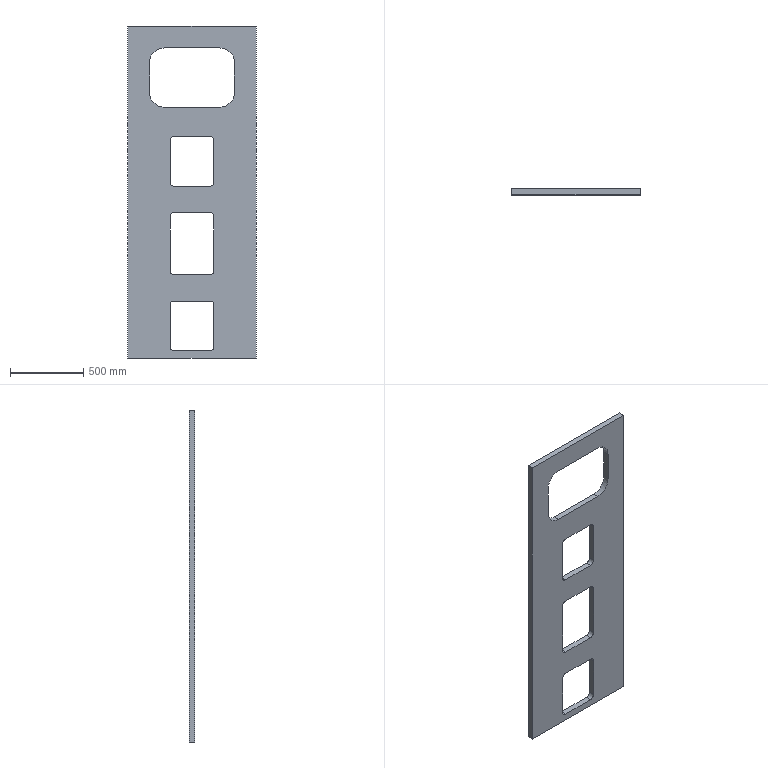Part | SolidWorks | features Cut 4, Fillet 2, Extrusion 1 | 1 solid | 38 faces | box 880 x 40 x 2266 mm | volume 57536483 mm3 | plane 22 | cylinder 16 | commonest cylinder face diameters 60 x12 200 x4
STEP:
#1=CARTESIAN_POINT('',(440.,0.,1133.));
#2=VERTEX_POINT('',#1);
#3=CARTESIAN_POINT('',(440.,0.,-1133.));
#4=VERTEX_POINT('',#3);
#5=CARTESIAN_POINT('',(440.,0.,1133.));
#6=DIRECTION('',(0.,0.,-1.));
#7=VECTOR('',#6,1000.);
#8=LINE('',#5,#7);
#9=EDGE_CURVE('',#2,#4,#8,.T.);
#10=ORIENTED_EDGE('',*,*,#9,.T.);
#11=CARTESIAN_POINT('',(440.,40.,-1133.));
#12=VERTEX_POINT('',#11);
#13=CARTESIAN_POINT('',(440.,40.,-1133.));
#14=DIRECTION('',(0.,-1.,0.));
#15=VECTOR('',#14,1000.);
#16=LINE('',#13,#15);
#17=EDGE_CURVE('',#12,#4,#16,.T.);
#18=ORIENTED_EDGE('',*,*,#17,.F.);
#19=CARTESIAN_POINT('',(440.,40.,1133.));
#20=VERTEX_POINT('',#19);
#21=CARTESIAN_POINT('',(440.,40.,1133.));
#22=DIRECTION('',(0.,0.,-1.));
#23=VECTOR('',#22,1000.);
#24=LINE('',#21,#23);
#25=EDGE_CURVE('',#20,#12,#24,.T.);
#26=ORIENTED_EDGE('',*,*,#25,.F.);
#27=CARTESIAN_POINT('',(440.,40.,1133.));
#28=DIRECTION('',(0.,-1.,0.));
#29=VECTOR('',#28,1000.);
#30=LINE('',#27,#29);
#31=EDGE_CURVE('',#20,#2,#30,.T.);
#32=ORIENTED_EDGE('',*,*,#31,.T.);
#33=EDGE_LOOP('',(#10,#18,#26,#32));
#34=FACE_OUTER_BOUND('',#33,.T.);
#35=CARTESIAN_POINT('',(440.,40.,1133.));
#36=DIRECTION('',(-1.,0.,0.));
#37=DIRECTION('',(0.,0.,1.));
#38=AXIS2_PLACEMENT_3D('',#35,#36,#37);
#39=PLANE('',#38);
#40=ADVANCED_FACE('',(#34),#39,.F.);
#41=CARTESIAN_POINT('',(-440.,0.,-1133.));
#42=VERTEX_POINT('',#41);
#43=CARTESIAN_POINT('',(-440.,0.,-1133.));
#44=DIRECTION('',(-1.,0.,0.));
#45=VECTOR('',#44,1000.);
#46=LINE('',#43,#45);
#47=EDGE_CURVE('',#4,#42,#46,.T.);
#48=ORIENTED_EDGE('',*,*,#47,.T.);
#49=CARTESIAN_POINT('',(-440.,40.,-1133.));
#50=VERTEX_POINT('',#49);
#51=CARTESIAN_POINT('',(-440.,40.,-1133.));
#52=DIRECTION('',(0.,-1.,0.));
#53=VECTOR('',#52,1000.);
#54=LINE('',#51,#53);
#55=EDGE_CURVE('',#50,#42,#54,.T.);
#56=ORIENTED_EDGE('',*,*,#55,.F.);
#57=CARTESIAN_POINT('',(-440.,40.,-1133.));
#58=DIRECTION('',(-1.,0.,0.));
#59=VECTOR('',#58,1000.);
#60=LINE('',#57,#59);
#61=EDGE_CURVE('',#12,#50,#60,.T.);
#62=ORIENTED_EDGE('',*,*,#61,.F.);
#63=ORIENTED_EDGE('',*,*,#17,.T.);
#64=EDGE_LOOP('',(#48,#56,#62,#63));
#65=FACE_OUTER_BOUND('',#64,.T.);
#66=CARTESIAN_POINT('',(-440.,40.,-1133.));
#67=DIRECTION('',(0.,0.,1.));
#68=DIRECTION('',(1.,0.,0.));
#69=AXIS2_PLACEMENT_3D('',#66,#67,#68);
#70=PLANE('',#69);
#71=ADVANCED_FACE('',(#65),#70,.F.);
#72=CARTESIAN_POINT('',(-440.,0.,1133.));
#73=VERTEX_POINT('',#72);
#74=CARTESIAN_POINT('',(-440.,0.,1133.));
#75=DIRECTION('',(0.,0.,1.));
#76=VECTOR('',#75,1000.);
#77=LINE('',#74,#76);
#78=EDGE_CURVE('',#42,#73,#77,.T.);
#79=ORIENTED_EDGE('',*,*,#78,.T.);
#80=CARTESIAN_POINT('',(-440.,40.,1133.));
#81=VERTEX_POINT('',#80);
#82=CARTESIAN_POINT('',(-440.,40.,1133.));
#83=DIRECTION('',(0.,-1.,0.));
#84=VECTOR('',#83,1000.);
#85=LINE('',#82,#84);
#86=EDGE_CURVE('',#81,#73,#85,.T.);
#87=ORIENTED_EDGE('',*,*,#86,.F.);
#88=CARTESIAN_POINT('',(-440.,40.,1133.));
#89=DIRECTION('',(0.,0.,1.));
#90=VECTOR('',#89,1000.);
#91=LINE('',#88,#90);
#92=EDGE_CURVE('',#50,#81,#91,.T.);
#93=ORIENTED_EDGE('',*,*,#92,.F.);
#94=ORIENTED_EDGE('',*,*,#55,.T.);
#95=EDGE_LOOP('',(#79,#87,#93,#94));
#96=FACE_OUTER_BOUND('',#95,.T.);
#97=CARTESIAN_POINT('',(-440.,40.,1133.));
#98=DIRECTION('',(1.,0.,0.));
#99=DIRECTION('',(0.,0.,-1.));
#100=AXIS2_PLACEMENT_3D('',#97,#98,#99);
#101=PLANE('',#100);
#102=ADVANCED_FACE('',(#96),#101,.F.);
#103=CARTESIAN_POINT('',(-440.,0.,1133.));
#104=DIRECTION('',(1.,0.,0.));
#105=VECTOR('',#104,1000.);
#106=LINE('',#103,#105);
#107=EDGE_CURVE('',#73,#2,#106,.T.);
#108=ORIENTED_EDGE('',*,*,#107,.T.);
#109=ORIENTED_EDGE('',*,*,#31,.F.);
#110=CARTESIAN_POINT('',(-440.,40.,1133.));
#111=DIRECTION('',(1.,0.,0.));
#112=VECTOR('',#111,1000.);
#113=LINE('',#110,#112);
#114=EDGE_CURVE('',#81,#20,#113,.T.);
#115=ORIENTED_EDGE('',*,*,#114,.F.);
#116=ORIENTED_EDGE('',*,*,#86,.T.);
#117=EDGE_LOOP('',(#108,#109,#115,#116));
#118=FACE_OUTER_BOUND('',#117,.T.);
#119=CARTESIAN_POINT('',(-440.,40.,1133.));
#120=DIRECTION('',(0.,0.,-1.));
#121=DIRECTION('',(-1.,0.,0.));
#122=AXIS2_PLACEMENT_3D('',#119,#120,#121);
#123=PLANE('',#122);
#124=ADVANCED_FACE('',(#118),#123,.F.);
#125=CARTESIAN_POINT('',(290.,40.,678.985));
#126=VERTEX_POINT('',#125);
#127=CARTESIAN_POINT('',(290.,40.,883.));
#128=VERTEX_POINT('',#127);
#129=CARTESIAN_POINT('',(290.,40.,983.));
#130=DIRECTION('',(0.,0.,1.));
#131=VECTOR('',#130,1000.);
#132=LINE('',#129,#131);
#133=EDGE_CURVE('',#126,#128,#132,.T.);
#134=ORIENTED_EDGE('',*,*,#133,.T.);
#135=CARTESIAN_POINT('',(190.,40.,983.));
#136=VERTEX_POINT('',#135);
#137=CARTESIAN_POINT('',(190.,40.,883.));
#138=DIRECTION('',(0.,-1.,0.));
#139=DIRECTION('',(0.,0.,-1.));
#140=AXIS2_PLACEMENT_3D('',#137,#138,#139);
#141=CIRCLE('',#140,100.);
#142=EDGE_CURVE('',#128,#136,#141,.T.);
#143=ORIENTED_EDGE('',*,*,#142,.T.);
#144=CARTESIAN_POINT('',(-190.,40.,983.));
#145=VERTEX_POINT('',#144);
#146=CARTESIAN_POINT('',(-290.,40.,983.));
#147=DIRECTION('',(-1.,0.,0.));
#148=VECTOR('',#147,1000.);
#149=LINE('',#146,#148);
#150=EDGE_CURVE('',#136,#145,#149,.T.);
#151=ORIENTED_EDGE('',*,*,#150,.T.);
#152=CARTESIAN_POINT('',(-290.,40.,883.));
#153=VERTEX_POINT('',#152);
#154=CARTESIAN_POINT('',(-190.,40.,883.));
#155=DIRECTION('',(0.,-1.,0.));
#156=DIRECTION('',(0.,0.,-1.));
#157=AXIS2_PLACEMENT_3D('',#154,#155,#156);
#158=CIRCLE('',#157,100.);
#159=EDGE_CURVE('',#145,#153,#158,.T.);
#160=ORIENTED_EDGE('',*,*,#159,.T.);
#161=CARTESIAN_POINT('',(-290.,40.,678.985));
#162=VERTEX_POINT('',#161);
#163=CARTESIAN_POINT('',(-290.,40.,983.));
#164=DIRECTION('',(0.,0.,-1.));
#165=VECTOR('',#164,1000.);
#166=LINE('',#163,#165);
#167=EDGE_CURVE('',#153,#162,#166,.T.);
#168=ORIENTED_EDGE('',*,*,#167,.T.);
#169=CARTESIAN_POINT('',(-190.,40.,578.985));
#170=VERTEX_POINT('',#169);
#171=CARTESIAN_POINT('',(-190.,40.,678.985));
#172=DIRECTION('',(0.,-1.,0.));
#173=DIRECTION('',(0.,0.,-1.));
#174=AXIS2_PLACEMENT_3D('',#171,#172,#173);
#175=CIRCLE('',#174,100.);
#176=EDGE_CURVE('',#162,#170,#175,.T.);
#177=ORIENTED_EDGE('',*,*,#176,.T.);
#178=CARTESIAN_POINT('',(190.,40.,578.985));
#179=VERTEX_POINT('',#178);
#180=CARTESIAN_POINT('',(-290.,40.,578.985));
#181=DIRECTION('',(1.,0.,0.));
#182=VECTOR('',#181,1000.);
#183=LINE('',#180,#182);
#184=EDGE_CURVE('',#170,#179,#183,.T.);
#185=ORIENTED_EDGE('',*,*,#184,.T.);
#186=CARTESIAN_POINT('',(190.,40.,678.985));
#187=DIRECTION('',(0.,-1.,0.));
#188=DIRECTION('',(0.,0.,-1.));
#189=AXIS2_PLACEMENT_3D('',#186,#187,#188);
#190=CIRCLE('',#189,100.);
#191=EDGE_CURVE('',#179,#126,#190,.T.);
#192=ORIENTED_EDGE('',*,*,#191,.T.);
#193=EDGE_LOOP('',(#134,#143,#151,#160,#168,#177,#185,#192));
#194=FACE_BOUND('',#193,.T.);
#195=CARTESIAN_POINT('',(150.,40.,-1054.485));
#196=VERTEX_POINT('',#195);
#197=CARTESIAN_POINT('',(150.,40.,-774.015));
#198=VERTEX_POINT('',#197);
#199=CARTESIAN_POINT('',(150.,40.,-744.015));
#200=DIRECTION('',(0.,0.,1.));
#201=VECTOR('',#200,1000.);
#202=LINE('',#199,#201);
#203=EDGE_CURVE('',#196,#198,#202,.T.);
#204=ORIENTED_EDGE('',*,*,#203,.T.);
#205=CARTESIAN_POINT('',(120.,40.,-744.015));
#206=VERTEX_POINT('',#205);
#207=CARTESIAN_POINT('',(120.,40.,-774.015));
#208=DIRECTION('',(0.,-1.,0.));
#209=DIRECTION('',(0.,0.,-1.));
#210=AXIS2_PLACEMENT_3D('',#207,#208,#209);
#211=CIRCLE('',#210,30.);
#212=EDGE_CURVE('',#198,#206,#211,.T.);
#213=ORIENTED_EDGE('',*,*,#212,.T.);
#214=CARTESIAN_POINT('',(-120.,40.,-744.015));
#215=VERTEX_POINT('',#214);
#216=CARTESIAN_POINT('',(-150.,40.,-744.015));
#217=DIRECTION('',(-1.,0.,0.));
#218=VECTOR('',#217,1000.);
#219=LINE('',#216,#218);
#220=EDGE_CURVE('',#206,#215,#219,.T.);
#221=ORIENTED_EDGE('',*,*,#220,.T.);
#222=CARTESIAN_POINT('',(-150.,40.,-774.015));
#223=VERTEX_POINT('',#222);
#224=CARTESIAN_POINT('',(-120.,40.,-774.015));
#225=DIRECTION('',(0.,-1.,0.));
#226=DIRECTION('',(0.,0.,-1.));
#227=AXIS2_PLACEMENT_3D('',#224,#225,#226);
#228=CIRCLE('',#227,30.);
#229=EDGE_CURVE('',#215,#223,#228,.T.);
#230=ORIENTED_EDGE('',*,*,#229,.T.);
#231=CARTESIAN_POINT('',(-150.,40.,-1054.485));
#232=VERTEX_POINT('',#231);
#233=CARTESIAN_POINT('',(-150.,40.,-744.015));
#234=DIRECTION('',(0.,0.,-1.));
#235=VECTOR('',#234,1000.);
#236=LINE('',#233,#235);
#237=EDGE_CURVE('',#223,#232,#236,.T.);
#238=ORIENTED_EDGE('',*,*,#237,.T.);
#239=CARTESIAN_POINT('',(-120.,40.,-1084.485));
#240=VERTEX_POINT('',#239);
#241=CARTESIAN_POINT('',(-120.,40.,-1054.485));
#242=DIRECTION('',(0.,-1.,0.));
#243=DIRECTION('',(0.,0.,-1.));
#244=AXIS2_PLACEMENT_3D('',#241,#242,#243);
#245=CIRCLE('',#244,30.);
#246=EDGE_CURVE('',#232,#240,#245,.T.);
#247=ORIENTED_EDGE('',*,*,#246,.T.);
#248=CARTESIAN_POINT('',(120.,40.,-1084.485));
#249=VERTEX_POINT('',#248);
#250=CARTESIAN_POINT('',(-150.,40.,-1084.485));
#251=DIRECTION('',(1.,0.,0.));
#252=VECTOR('',#251,1000.);
#253=LINE('',#250,#252);
#254=EDGE_CURVE('',#240,#249,#253,.T.);
#255=ORIENTED_EDGE('',*,*,#254,.T.);
#256=CARTESIAN_POINT('',(120.,40.,-1054.485));
#257=DIRECTION('',(0.,-1.,0.));
#258=DIRECTION('',(0.,0.,-1.));
#259=AXIS2_PLACEMENT_3D('',#256,#257,#258);
#260=CIRCLE('',#259,30.);
#261=EDGE_CURVE('',#249,#196,#260,.T.);
#262=ORIENTED_EDGE('',*,*,#261,.T.);
#263=EDGE_LOOP('',(#204,#213,#221,#230,#238,#247,#255,#262));
#264=FACE_BOUND('',#263,.T.);
#265=CARTESIAN_POINT('',(150.,40.,-536.015));
#266=VERTEX_POINT('',#265);
#267=CARTESIAN_POINT('',(150.,40.,-169.485));
#268=VERTEX_POINT('',#267);
#269=CARTESIAN_POINT('',(150.,40.,-566.015));
#270=DIRECTION('',(0.,0.,1.));
#271=VECTOR('',#270,1000.);
#272=LINE('',#269,#271);
#273=EDGE_CURVE('',#266,#268,#272,.T.);
#274=ORIENTED_EDGE('',*,*,#273,.T.);
#275=CARTESIAN_POINT('',(120.,40.,-139.485));
#276=VERTEX_POINT('',#275);
#277=CARTESIAN_POINT('',(120.,40.,-169.485));
#278=DIRECTION('',(0.,-1.,0.));
#279=DIRECTION('',(0.,0.,-1.));
#280=AXIS2_PLACEMENT_3D('',#277,#278,#279);
#281=CIRCLE('',#280,30.);
#282=EDGE_CURVE('',#268,#276,#281,.T.);
#283=ORIENTED_EDGE('',*,*,#282,.T.);
#284=CARTESIAN_POINT('',(-120.,40.,-139.485));
#285=VERTEX_POINT('',#284);
#286=CARTESIAN_POINT('',(-150.,40.,-139.485));
#287=DIRECTION('',(-1.,0.,0.));
#288=VECTOR('',#287,1000.);
#289=LINE('',#286,#288);
#290=EDGE_CURVE('',#276,#285,#289,.T.);
#291=ORIENTED_EDGE('',*,*,#290,.T.);
#292=CARTESIAN_POINT('',(-150.,40.,-169.485));
#293=VERTEX_POINT('',#292);
#294=CARTESIAN_POINT('',(-120.,40.,-169.485));
#295=DIRECTION('',(0.,-1.,0.));
#296=DIRECTION('',(0.,0.,-1.));
#297=AXIS2_PLACEMENT_3D('',#294,#295,#296);
#298=CIRCLE('',#297,30.);
#299=EDGE_CURVE('',#285,#293,#298,.T.);
#300=ORIENTED_EDGE('',*,*,#299,.T.);
#301=CARTESIAN_POINT('',(-150.,40.,-536.015));
#302=VERTEX_POINT('',#301);
#303=CARTESIAN_POINT('',(-150.,40.,-566.015));
#304=DIRECTION('',(0.,0.,-1.));
#305=VECTOR('',#304,1000.);
#306=LINE('',#303,#305);
#307=EDGE_CURVE('',#293,#302,#306,.T.);
#308=ORIENTED_EDGE('',*,*,#307,.T.);
#309=CARTESIAN_POINT('',(-120.,40.,-566.015));
#310=VERTEX_POINT('',#309);
#311=CARTESIAN_POINT('',(-120.,40.,-536.015));
#312=DIRECTION('',(0.,-1.,0.));
#313=DIRECTION('',(0.,0.,-1.));
#314=AXIS2_PLACEMENT_3D('',#311,#312,#313);
#315=CIRCLE('',#314,30.);
#316=EDGE_CURVE('',#302,#310,#315,.T.);
#317=ORIENTED_EDGE('',*,*,#316,.T.);
#318=CARTESIAN_POINT('',(120.,40.,-566.015));
#319=VERTEX_POINT('',#318);
#320=CARTESIAN_POINT('',(-150.,40.,-566.015));
#321=DIRECTION('',(1.,0.,0.));
#322=VECTOR('',#321,1000.);
#323=LINE('',#320,#322);
#324=EDGE_CURVE('',#310,#319,#323,.T.);
#325=ORIENTED_EDGE('',*,*,#324,.T.);
#326=CARTESIAN_POINT('',(120.,40.,-536.015));
#327=DIRECTION('',(0.,-1.,0.));
#328=DIRECTION('',(0.,0.,-1.));
#329=AXIS2_PLACEMENT_3D('',#326,#327,#328);
#330=CIRCLE('',#329,30.);
#331=EDGE_CURVE('',#319,#266,#330,.T.);
#332=ORIENTED_EDGE('',*,*,#331,.T.);
#333=EDGE_LOOP('',(#274,#283,#291,#300,#308,#317,#325,#332));
#334=FACE_BOUND('',#333,.T.);
#335=CARTESIAN_POINT('',(150.,40.,68.515));
#336=VERTEX_POINT('',#335);
#337=CARTESIAN_POINT('',(150.,40.,348.985));
#338=VERTEX_POINT('',#337);
#339=CARTESIAN_POINT('',(150.,40.,378.985));
#340=DIRECTION('',(0.,0.,1.));
#341=VECTOR('',#340,1000.);
#342=LINE('',#339,#341);
#343=EDGE_CURVE('',#336,#338,#342,.T.);
#344=ORIENTED_EDGE('',*,*,#343,.T.);
#345=CARTESIAN_POINT('',(120.,40.,378.985));
#346=VERTEX_POINT('',#345);
#347=CARTESIAN_POINT('',(120.,40.,348.985));
#348=DIRECTION('',(0.,-1.,0.));
#349=DIRECTION('',(0.,0.,-1.));
#350=AXIS2_PLACEMENT_3D('',#347,#348,#349);
#351=CIRCLE('',#350,30.);
#352=EDGE_CURVE('',#338,#346,#351,.T.);
#353=ORIENTED_EDGE('',*,*,#352,.T.);
#354=CARTESIAN_POINT('',(-120.,40.,378.985));
#355=VERTEX_POINT('',#354);
#356=CARTESIAN_POINT('',(-150.,40.,378.985));
#357=DIRECTION('',(-1.,0.,0.));
#358=VECTOR('',#357,1000.);
#359=LINE('',#356,#358);
#360=EDGE_CURVE('',#346,#355,#359,.T.);
#361=ORIENTED_EDGE('',*,*,#360,.T.);
#362=CARTESIAN_POINT('',(-150.,40.,348.985));
#363=VERTEX_POINT('',#362);
#364=CARTESIAN_POINT('',(-120.,40.,348.985));
#365=DIRECTION('',(0.,-1.,0.));
#366=DIRECTION('',(0.,0.,-1.));
#367=AXIS2_PLACEMENT_3D('',#364,#365,#366);
#368=CIRCLE('',#367,30.);
#369=EDGE_CURVE('',#355,#363,#368,.T.);
#370=ORIENTED_EDGE('',*,*,#369,.T.);
#371=CARTESIAN_POINT('',(-150.,40.,68.515));
#372=VERTEX_POINT('',#371);
#373=CARTESIAN_POINT('',(-150.,40.,378.985));
#374=DIRECTION('',(0.,0.,-1.));
#375=VECTOR('',#374,1000.);
#376=LINE('',#373,#375);
#377=EDGE_CURVE('',#363,#372,#376,.T.);
#378=ORIENTED_EDGE('',*,*,#377,.T.);
#379=CARTESIAN_POINT('',(-120.,40.,38.515));
#380=VERTEX_POINT('',#379);
#381=CARTESIAN_POINT('',(-120.,40.,68.515));
#382=DIRECTION('',(0.,-1.,0.));
#383=DIRECTION('',(0.,0.,-1.));
#384=AXIS2_PLACEMENT_3D('',#381,#382,#383);
#385=CIRCLE('',#384,30.);
#386=EDGE_CURVE('',#372,#380,#385,.T.);
#387=ORIENTED_EDGE('',*,*,#386,.T.);
#388=CARTESIAN_POINT('',(120.,40.,38.515));
#389=VERTEX_POINT('',#388);
#390=CARTESIAN_POINT('',(-150.,40.,38.515));
#391=DIRECTION('',(1.,0.,0.));
#392=VECTOR('',#391,1000.);
#393=LINE('',#390,#392);
#394=EDGE_CURVE('',#380,#389,#393,.T.);
#395=ORIENTED_EDGE('',*,*,#394,.T.);
#396=CARTESIAN_POINT('',(120.,40.,68.515));
#397=DIRECTION('',(0.,-1.,0.));
#398=DIRECTION('',(0.,0.,-1.));
#399=AXIS2_PLACEMENT_3D('',#396,#397,#398);
#400=CIRCLE('',#399,30.);
#401=EDGE_CURVE('',#389,#336,#400,.T.);
#402=ORIENTED_EDGE('',*,*,#401,.T.);
#403=EDGE_LOOP('',(#344,#353,#361,#370,#378,#387,#395,#402));
#404=FACE_BOUND('',#403,.T.);
#405=ORIENTED_EDGE('',*,*,#25,.T.);
#406=ORIENTED_EDGE('',*,*,#61,.T.);
#407=ORIENTED_EDGE('',*,*,#92,.T.);
#408=ORIENTED_EDGE('',*,*,#114,.T.);
#409=EDGE_LOOP('',(#405,#406,#407,#408));
#410=FACE_OUTER_BOUND('',#409,.T.);
#411=CARTESIAN_POINT('',(0.,40.,0.));
#412=DIRECTION('',(0.,-1.,0.));
#413=DIRECTION('',(0.,0.,-1.));
#414=AXIS2_PLACEMENT_3D('',#411,#412,#413);
#415=PLANE('',#414);
#416=ADVANCED_FACE('',(#194,#264,#334,#404,#410),#415,.F.);
#417=CARTESIAN_POINT('',(-290.,0.,883.));
#418=VERTEX_POINT('',#417);
#419=CARTESIAN_POINT('',(-290.,0.,678.985));
#420=VERTEX_POINT('',#419);
#421=CARTESIAN_POINT('',(-290.,0.,983.));
#422=DIRECTION('',(0.,0.,-1.));
#423=VECTOR('',#422,1000.);
#424=LINE('',#421,#423);
#425=EDGE_CURVE('',#418,#420,#424,.T.);
#426=ORIENTED_EDGE('',*,*,#425,.F.);
#427=CARTESIAN_POINT('',(-190.,0.,983.));
#428=VERTEX_POINT('',#427);
#429=CARTESIAN_POINT('',(-190.,0.,883.));
#430=DIRECTION('',(0.,1.,0.));
#431=DIRECTION('',(0.,0.,-1.));
#432=AXIS2_PLACEMENT_3D('',#429,#430,#431);
#433=CIRCLE('',#432,100.);
#434=EDGE_CURVE('',#418,#428,#433,.T.);
#435=ORIENTED_EDGE('',*,*,#434,.T.);
#436=CARTESIAN_POINT('',(190.,0.,983.));
#437=VERTEX_POINT('',#436);
#438=CARTESIAN_POINT('',(-290.,0.,983.));
#439=DIRECTION('',(-1.,0.,0.));
#440=VECTOR('',#439,1000.);
#441=LINE('',#438,#440);
#442=EDGE_CURVE('',#437,#428,#441,.T.);
#443=ORIENTED_EDGE('',*,*,#442,.F.);
#444=CARTESIAN_POINT('',(290.,0.,883.));
#445=VERTEX_POINT('',#444);
#446=CARTESIAN_POINT('',(190.,0.,883.));
#447=DIRECTION('',(0.,1.,0.));
#448=DIRECTION('',(0.,0.,-1.));
#449=AXIS2_PLACEMENT_3D('',#446,#447,#448);
#450=CIRCLE('',#449,100.);
#451=EDGE_CURVE('',#437,#445,#450,.T.);
#452=ORIENTED_EDGE('',*,*,#451,.T.);
#453=CARTESIAN_POINT('',(290.,0.,678.985));
#454=VERTEX_POINT('',#453);
#455=CARTESIAN_POINT('',(290.,0.,983.));
#456=DIRECTION('',(0.,0.,1.));
#457=VECTOR('',#456,1000.);
#458=LINE('',#455,#457);
#459=EDGE_CURVE('',#454,#445,#458,.T.);
#460=ORIENTED_EDGE('',*,*,#459,.F.);
#461=CARTESIAN_POINT('',(190.,0.,578.985));
#462=VERTEX_POINT('',#461);
#463=CARTESIAN_POINT('',(190.,0.,678.985));
#464=DIRECTION('',(0.,1.,0.));
#465=DIRECTION('',(0.,0.,-1.));
#466=AXIS2_PLACEMENT_3D('',#463,#464,#465);
#467=CIRCLE('',#466,100.);
#468=EDGE_CURVE('',#454,#462,#467,.T.);
#469=ORIENTED_EDGE('',*,*,#468,.T.);
#470=CARTESIAN_POINT('',(-190.,0.,578.985));
#471=VERTEX_POINT('',#470);
#472=CARTESIAN_POINT('',(-290.,0.,578.985));
#473=DIRECTION('',(1.,0.,0.));
#474=VECTOR('',#473,1000.);
#475=LINE('',#472,#474);
#476=EDGE_CURVE('',#471,#462,#475,.T.);
#477=ORIENTED_EDGE('',*,*,#476,.F.);
#478=CARTESIAN_POINT('',(-190.,0.,678.985));
#479=DIRECTION('',(0.,1.,0.));
#480=DIRECTION('',(0.,0.,-1.));
#481=AXIS2_PLACEMENT_3D('',#478,#479,#480);
#482=CIRCLE('',#481,100.);
#483=EDGE_CURVE('',#471,#420,#482,.T.);
#484=ORIENTED_EDGE('',*,*,#483,.T.);
#485=EDGE_LOOP('',(#426,#435,#443,#452,#460,#469,#477,#484));
#486=FACE_BOUND('',#485,.T.);
#487=CARTESIAN_POINT('',(-150.,0.,-774.015));
#488=VERTEX_POINT('',#487);
#489=CARTESIAN_POINT('',(-150.,0.,-1054.485));
#490=VERTEX_POINT('',#489);
#491=CARTESIAN_POINT('',(-150.,0.,-744.015));
#492=DIRECTION('',(0.,0.,-1.));
#493=VECTOR('',#492,1000.);
#494=LINE('',#491,#493);
#495=EDGE_CURVE('',#488,#490,#494,.T.);
#496=ORIENTED_EDGE('',*,*,#495,.F.);
#497=CARTESIAN_POINT('',(-120.,0.,-744.015));
#498=VERTEX_POINT('',#497);
#499=CARTESIAN_POINT('',(-120.,0.,-774.015));
#500=DIRECTION('',(0.,1.,0.));
#501=DIRECTION('',(0.,0.,-1.));
#502=AXIS2_PLACEMENT_3D('',#499,#500,#501);
#503=CIRCLE('',#502,30.);
#504=EDGE_CURVE('',#488,#498,#503,.T.);
#505=ORIENTED_EDGE('',*,*,#504,.T.);
#506=CARTESIAN_POINT('',(120.,0.,-744.015));
#507=VERTEX_POINT('',#506);
#508=CARTESIAN_POINT('',(-150.,0.,-744.015));
#509=DIRECTION('',(-1.,0.,0.));
#510=VECTOR('',#509,1000.);
#511=LINE('',#508,#510);
#512=EDGE_CURVE('',#507,#498,#511,.T.);
#513=ORIENTED_EDGE('',*,*,#512,.F.);
#514=CARTESIAN_POINT('',(150.,0.,-774.015));
#515=VERTEX_POINT('',#514);
#516=CARTESIAN_POINT('',(120.,0.,-774.015));
#517=DIRECTION('',(0.,1.,0.));
#518=DIRECTION('',(0.,0.,-1.));
#519=AXIS2_PLACEMENT_3D('',#516,#517,#518);
#520=CIRCLE('',#519,30.);
#521=EDGE_CURVE('',#507,#515,#520,.T.);
#522=ORIENTED_EDGE('',*,*,#521,.T.);
#523=CARTESIAN_POINT('',(150.,0.,-1054.485));
#524=VERTEX_POINT('',#523);
#525=CARTESIAN_POINT('',(150.,0.,-744.015));
#526=DIRECTION('',(0.,0.,1.));
#527=VECTOR('',#526,1000.);
#528=LINE('',#525,#527);
#529=EDGE_CURVE('',#524,#515,#528,.T.);
#530=ORIENTED_EDGE('',*,*,#529,.F.);
#531=CARTESIAN_POINT('',(120.,0.,-1084.485));
#532=VERTEX_POINT('',#531);
#533=CARTESIAN_POINT('',(120.,0.,-1054.485));
#534=DIRECTION('',(0.,1.,0.));
#535=DIRECTION('',(0.,0.,-1.));
#536=AXIS2_PLACEMENT_3D('',#533,#534,#535);
#537=CIRCLE('',#536,30.);
#538=EDGE_CURVE('',#524,#532,#537,.T.);
#539=ORIENTED_EDGE('',*,*,#538,.T.);
#540=CARTESIAN_POINT('',(-120.,0.,-1084.485));
#541=VERTEX_POINT('',#540);
#542=CARTESIAN_POINT('',(-150.,0.,-1084.485));
#543=DIRECTION('',(1.,0.,0.));
#544=VECTOR('',#543,1000.);
#545=LINE('',#542,#544);
#546=EDGE_CURVE('',#541,#532,#545,.T.);
#547=ORIENTED_EDGE('',*,*,#546,.F.);
#548=CARTESIAN_POINT('',(-120.,0.,-1054.485));
#549=DIRECTION('',(0.,1.,0.));
#550=DIRECTION('',(0.,0.,-1.));
#551=AXIS2_PLACEMENT_3D('',#548,#549,#550);
#552=CIRCLE('',#551,30.);
#553=EDGE_CURVE('',#541,#490,#552,.T.);
#554=ORIENTED_EDGE('',*,*,#553,.T.);
#555=EDGE_LOOP('',(#496,#505,#513,#522,#530,#539,#547,#554));
#556=FACE_BOUND('',#555,.T.);
#557=CARTESIAN_POINT('',(-150.,0.,-169.485));
#558=VERTEX_POINT('',#557);
#559=CARTESIAN_POINT('',(-150.,0.,-536.015));
#560=VERTEX_POINT('',#559);
#561=CARTESIAN_POINT('',(-150.,0.,-566.015));
#562=DIRECTION('',(0.,0.,-1.));
#563=VECTOR('',#562,1000.);
#564=LINE('',#561,#563);
#565=EDGE_CURVE('',#558,#560,#564,.T.);
#566=ORIENTED_EDGE('',*,*,#565,.F.);
#567=CARTESIAN_POINT('',(-120.,0.,-139.485));
#568=VERTEX_POINT('',#567);
#569=CARTESIAN_POINT('',(-120.,0.,-169.485));
#570=DIRECTION('',(0.,1.,0.));
#571=DIRECTION('',(0.,0.,-1.));
#572=AXIS2_PLACEMENT_3D('',#569,#570,#571);
#573=CIRCLE('',#572,30.);
#574=EDGE_CURVE('',#558,#568,#573,.T.);
#575=ORIENTED_EDGE('',*,*,#574,.T.);
#576=CARTESIAN_POINT('',(120.,0.,-139.485));
#577=VERTEX_POINT('',#576);
#578=CARTESIAN_POINT('',(-150.,0.,-139.485));
#579=DIRECTION('',(-1.,0.,0.));
#580=VECTOR('',#579,1000.);
#581=LINE('',#578,#580);
#582=EDGE_CURVE('',#577,#568,#581,.T.);
#583=ORIENTED_EDGE('',*,*,#582,.F.);
#584=CARTESIAN_POINT('',(150.,0.,-169.485));
#585=VERTEX_POINT('',#584);
#586=CARTESIAN_POINT('',(120.,0.,-169.485));
#587=DIRECTION('',(0.,1.,0.));
#588=DIRECTION('',(0.,0.,-1.));
#589=AXIS2_PLACEMENT_3D('',#586,#587,#588);
#590=CIRCLE('',#589,30.);
#591=EDGE_CURVE('',#577,#585,#590,.T.);
#592=ORIENTED_EDGE('',*,*,#591,.T.);
#593=CARTESIAN_POINT('',(150.,0.,-536.015));
#594=VERTEX_POINT('',#593);
#595=CARTESIAN_POINT('',(150.,0.,-566.015));
#596=DIRECTION('',(0.,0.,1.));
#597=VECTOR('',#596,1000.);
#598=LINE('',#595,#597);
#599=EDGE_CURVE('',#594,#585,#598,.T.);
#600=ORIENTED_EDGE('',*,*,#599,.F.);
#601=CARTESIAN_POINT('',(120.,0.,-566.015));
#602=VERTEX_POINT('',#601);
#603=CARTESIAN_POINT('',(120.,0.,-536.015));
#604=DIRECTION('',(0.,1.,0.));
#605=DIRECTION('',(0.,0.,-1.));
#606=AXIS2_PLACEMENT_3D('',#603,#604,#605);
#607=CIRCLE('',#606,30.);
#608=EDGE_CURVE('',#594,#602,#607,.T.);
#609=ORIENTED_EDGE('',*,*,#608,.T.);
#610=CARTESIAN_POINT('',(-120.,0.,-566.015));
#611=VERTEX_POINT('',#610);
#612=CARTESIAN_POINT('',(-150.,0.,-566.015));
#613=DIRECTION('',(1.,0.,0.));
#614=VECTOR('',#613,1000.);
#615=LINE('',#612,#614);
#616=EDGE_CURVE('',#611,#602,#615,.T.);
#617=ORIENTED_EDGE('',*,*,#616,.F.);
#618=CARTESIAN_POINT('',(-120.,0.,-536.015));
#619=DIRECTION('',(0.,1.,0.));
#620=DIRECTION('',(0.,0.,-1.));
#621=AXIS2_PLACEMENT_3D('',#618,#619,#620);
#622=CIRCLE('',#621,30.);
#623=EDGE_CURVE('',#611,#560,#622,.T.);
#624=ORIENTED_EDGE('',*,*,#623,.T.);
#625=EDGE_LOOP('',(#566,#575,#583,#592,#600,#609,#617,#624));
#626=FACE_BOUND('',#625,.T.);
#627=CARTESIAN_POINT('',(-150.,0.,348.985));
#628=VERTEX_POINT('',#627);
#629=CARTESIAN_POINT('',(-150.,0.,68.515));
#630=VERTEX_POINT('',#629);
#631=CARTESIAN_POINT('',(-150.,0.,378.985));
#632=DIRECTION('',(0.,0.,-1.));
#633=VECTOR('',#632,1000.);
#634=LINE('',#631,#633);
#635=EDGE_CURVE('',#628,#630,#634,.T.);
#636=ORIENTED_EDGE('',*,*,#635,.F.);
#637=CARTESIAN_POINT('',(-120.,0.,378.985));
#638=VERTEX_POINT('',#637);
#639=CARTESIAN_POINT('',(-120.,0.,348.985));
#640=DIRECTION('',(0.,1.,0.));
#641=DIRECTION('',(0.,0.,-1.));
#642=AXIS2_PLACEMENT_3D('',#639,#640,#641);
#643=CIRCLE('',#642,30.);
#644=EDGE_CURVE('',#628,#638,#643,.T.);
#645=ORIENTED_EDGE('',*,*,#644,.T.);
#646=CARTESIAN_POINT('',(120.,0.,378.985));
#647=VERTEX_POINT('',#646);
#648=CARTESIAN_POINT('',(-150.,0.,378.985));
#649=DIRECTION('',(-1.,0.,0.));
#650=VECTOR('',#649,1000.);
#651=LINE('',#648,#650);
#652=EDGE_CURVE('',#647,#638,#651,.T.);
#653=ORIENTED_EDGE('',*,*,#652,.F.);
#654=CARTESIAN_POINT('',(150.,0.,348.985));
#655=VERTEX_POINT('',#654);
#656=CARTESIAN_POINT('',(120.,0.,348.985));
#657=DIRECTION('',(0.,1.,0.));
#658=DIRECTION('',(0.,0.,-1.));
#659=AXIS2_PLACEMENT_3D('',#656,#657,#658);
#660=CIRCLE('',#659,30.);
#661=EDGE_CURVE('',#647,#655,#660,.T.);
#662=ORIENTED_EDGE('',*,*,#661,.T.);
#663=CARTESIAN_POINT('',(150.,0.,68.515));
#664=VERTEX_POINT('',#663);
#665=CARTESIAN_POINT('',(150.,0.,378.985));
#666=DIRECTION('',(0.,0.,1.));
#667=VECTOR('',#666,1000.);
#668=LINE('',#665,#667);
#669=EDGE_CURVE('',#664,#655,#668,.T.);
#670=ORIENTED_EDGE('',*,*,#669,.F.);
#671=CARTESIAN_POINT('',(120.,0.,38.515));
#672=VERTEX_POINT('',#671);
#673=CARTESIAN_POINT('',(120.,0.,68.515));
#674=DIRECTION('',(0.,1.,0.));
#675=DIRECTION('',(0.,0.,-1.));
#676=AXIS2_PLACEMENT_3D('',#673,#674,#675);
#677=CIRCLE('',#676,30.);
#678=EDGE_CURVE('',#664,#672,#677,.T.);
#679=ORIENTED_EDGE('',*,*,#678,.T.);
#680=CARTESIAN_POINT('',(-120.,0.,38.515));
#681=VERTEX_POINT('',#680);
#682=CARTESIAN_POINT('',(-150.,0.,38.515));
#683=DIRECTION('',(1.,0.,0.));
#684=VECTOR('',#683,1000.);
#685=LINE('',#682,#684);
#686=EDGE_CURVE('',#681,#672,#685,.T.);
#687=ORIENTED_EDGE('',*,*,#686,.F.);
#688=CARTESIAN_POINT('',(-120.,0.,68.515));
#689=DIRECTION('',(0.,1.,0.));
#690=DIRECTION('',(0.,0.,-1.));
#691=AXIS2_PLACEMENT_3D('',#688,#689,#690);
#692=CIRCLE('',#691,30.);
#693=EDGE_CURVE('',#681,#630,#692,.T.);
#694=ORIENTED_EDGE('',*,*,#693,.T.);
#695=EDGE_LOOP('',(#636,#645,#653,#662,#670,#679,#687,#694));
#696=FACE_BOUND('',#695,.T.);
#697=ORIENTED_EDGE('',*,*,#9,.F.);
#698=ORIENTED_EDGE('',*,*,#107,.F.);
#699=ORIENTED_EDGE('',*,*,#78,.F.);
#700=ORIENTED_EDGE('',*,*,#47,.F.);
#701=EDGE_LOOP('',(#697,#698,#699,#700));
#702=FACE_OUTER_BOUND('',#701,.T.);
#703=CARTESIAN_POINT('',(0.,0.,0.));
#704=DIRECTION('',(0.,-1.,0.));
#705=DIRECTION('',(0.,0.,-1.));
#706=AXIS2_PLACEMENT_3D('',#703,#704,#705);
#707=PLANE('',#706);
#708=ADVANCED_FACE('',(#486,#556,#626,#696,#702),#707,.T.);
#709=ORIENTED_EDGE('',*,*,#635,.T.);
#710=CARTESIAN_POINT('',(-150.,40.,68.515));
#711=DIRECTION('',(0.,1.,0.));
#712=VECTOR('',#711,1000.);
#713=LINE('',#710,#712);
#714=EDGE_CURVE('',#630,#372,#713,.T.);
#715=ORIENTED_EDGE('',*,*,#714,.T.);
#716=ORIENTED_EDGE('',*,*,#377,.F.);
#717=CARTESIAN_POINT('',(-150.,0.,348.985));
#718=DIRECTION('',(0.,-1.,0.));
#719=VECTOR('',#718,1000.);
#720=LINE('',#717,#719);
#721=EDGE_CURVE('',#363,#628,#720,.T.);
#722=ORIENTED_EDGE('',*,*,#721,.T.);
#723=EDGE_LOOP('',(#709,#715,#716,#722));
#724=FACE_OUTER_BOUND('',#723,.T.);
#725=CARTESIAN_POINT('',(-150.,40.,378.985));
#726=DIRECTION('',(-1.,0.,0.));
#727=DIRECTION('',(0.,0.,1.));
#728=AXIS2_PLACEMENT_3D('',#725,#726,#727);
#729=PLANE('',#728);
#730=ADVANCED_FACE('',(#724),#729,.F.);
#731=ORIENTED_EDGE('',*,*,#360,.F.);
#732=CARTESIAN_POINT('',(120.,0.,378.985));
#733=DIRECTION('',(0.,-1.,0.));
#734=VECTOR('',#733,1000.);
#735=LINE('',#732,#734);
#736=EDGE_CURVE('',#346,#647,#735,.T.);
#737=ORIENTED_EDGE('',*,*,#736,.T.);
#738=ORIENTED_EDGE('',*,*,#652,.T.);
#739=CARTESIAN_POINT('',(-120.,40.,378.985));
#740=DIRECTION('',(0.,1.,0.));
#741=VECTOR('',#740,1000.);
#742=LINE('',#739,#741);
#743=EDGE_CURVE('',#638,#355,#742,.T.);
#744=ORIENTED_EDGE('',*,*,#743,.T.);
#745=EDGE_LOOP('',(#731,#737,#738,#744));
#746=FACE_OUTER_BOUND('',#745,.T.);
#747=CARTESIAN_POINT('',(-150.,40.,378.985));
#748=DIRECTION('',(0.,0.,1.));
#749=DIRECTION('',(1.,0.,0.));
#750=AXIS2_PLACEMENT_3D('',#747,#748,#749);
#751=PLANE('',#750);
#752=ADVANCED_FACE('',(#746),#751,.F.);
#753=ORIENTED_EDGE('',*,*,#669,.T.);
#754=CARTESIAN_POINT('',(150.,40.,348.985));
#755=DIRECTION('',(0.,1.,0.));
#756=VECTOR('',#755,1000.);
#757=LINE('',#754,#756);
#758=EDGE_CURVE('',#655,#338,#757,.T.);
#759=ORIENTED_EDGE('',*,*,#758,.T.);
#760=ORIENTED_EDGE('',*,*,#343,.F.);
#761=CARTESIAN_POINT('',(150.,0.,68.515));
#762=DIRECTION('',(0.,-1.,0.));
#763=VECTOR('',#762,1000.);
#764=LINE('',#761,#763);
#765=EDGE_CURVE('',#336,#664,#764,.T.);
#766=ORIENTED_EDGE('',*,*,#765,.T.);
#767=EDGE_LOOP('',(#753,#759,#760,#766));
#768=FACE_OUTER_BOUND('',#767,.T.);
#769=CARTESIAN_POINT('',(150.,40.,378.985));
#770=DIRECTION('',(1.,0.,0.));
#771=DIRECTION('',(0.,0.,-1.));
#772=AXIS2_PLACEMENT_3D('',#769,#770,#771);
#773=PLANE('',#772);
#774=ADVANCED_FACE('',(#768),#773,.F.);
#775=ORIENTED_EDGE('',*,*,#686,.T.);
#776=CARTESIAN_POINT('',(120.,40.,38.515));
#777=DIRECTION('',(0.,1.,0.));
#778=VECTOR('',#777,1000.);
#779=LINE('',#776,#778);
#780=EDGE_CURVE('',#672,#389,#779,.T.);
#781=ORIENTED_EDGE('',*,*,#780,.T.);
#782=ORIENTED_EDGE('',*,*,#394,.F.);
#783=CARTESIAN_POINT('',(-120.,0.,38.515));
#784=DIRECTION('',(0.,-1.,0.));
#785=VECTOR('',#784,1000.);
#786=LINE('',#783,#785);
#787=EDGE_CURVE('',#380,#681,#786,.T.);
#788=ORIENTED_EDGE('',*,*,#787,.T.);
#789=EDGE_LOOP('',(#775,#781,#782,#788));
#790=FACE_OUTER_BOUND('',#789,.T.);
#791=CARTESIAN_POINT('',(-150.,40.,38.515));
#792=DIRECTION('',(0.,0.,-1.));
#793=DIRECTION('',(-1.,0.,0.));
#794=AXIS2_PLACEMENT_3D('',#791,#792,#793);
#795=PLANE('',#794);
#796=ADVANCED_FACE('',(#790),#795,.F.);
#797=ORIENTED_EDGE('',*,*,#565,.T.);
#798=CARTESIAN_POINT('',(-150.,40.,-536.015));
#799=DIRECTION('',(0.,1.,0.));
#800=VECTOR('',#799,1000.);
#801=LINE('',#798,#800);
#802=EDGE_CURVE('',#560,#302,#801,.T.);
#803=ORIENTED_EDGE('',*,*,#802,.T.);
#804=ORIENTED_EDGE('',*,*,#307,.F.);
#805=CARTESIAN_POINT('',(-150.,0.,-169.485));
#806=DIRECTION('',(0.,-1.,0.));
#807=VECTOR('',#806,1000.);
#808=LINE('',#805,#807);
#809=EDGE_CURVE('',#293,#558,#808,.T.);
#810=ORIENTED_EDGE('',*,*,#809,.T.);
#811=EDGE_LOOP('',(#797,#803,#804,#810));
#812=FACE_OUTER_BOUND('',#811,.T.);
#813=CARTESIAN_POINT('',(-150.,40.,-566.015));
#814=DIRECTION('',(-1.,0.,0.));
#815=DIRECTION('',(0.,0.,1.));
#816=AXIS2_PLACEMENT_3D('',#813,#814,#815);
#817=PLANE('',#816);
#818=ADVANCED_FACE('',(#812),#817,.F.);
#819=ORIENTED_EDGE('',*,*,#290,.F.);
#820=CARTESIAN_POINT('',(120.,0.,-139.485));
#821=DIRECTION('',(0.,-1.,0.));
#822=VECTOR('',#821,1000.);
#823=LINE('',#820,#822);
#824=EDGE_CURVE('',#276,#577,#823,.T.);
#825=ORIENTED_EDGE('',*,*,#824,.T.);
#826=ORIENTED_EDGE('',*,*,#582,.T.);
#827=CARTESIAN_POINT('',(-120.,40.,-139.485));
#828=DIRECTION('',(0.,1.,0.));
#829=VECTOR('',#828,1000.);
#830=LINE('',#827,#829);
#831=EDGE_CURVE('',#568,#285,#830,.T.);
#832=ORIENTED_EDGE('',*,*,#831,.T.);
#833=EDGE_LOOP('',(#819,#825,#826,#832));
#834=FACE_OUTER_BOUND('',#833,.T.);
#835=CARTESIAN_POINT('',(-150.,40.,-139.485));
#836=DIRECTION('',(0.,0.,1.));
#837=DIRECTION('',(1.,0.,0.));
#838=AXIS2_PLACEMENT_3D('',#835,#836,#837);
#839=PLANE('',#838);
#840=ADVANCED_FACE('',(#834),#839,.F.);
#841=ORIENTED_EDGE('',*,*,#599,.T.);
#842=CARTESIAN_POINT('',(150.,40.,-169.485));
#843=DIRECTION('',(0.,1.,0.));
#844=VECTOR('',#843,1000.);
#845=LINE('',#842,#844);
#846=EDGE_CURVE('',#585,#268,#845,.T.);
#847=ORIENTED_EDGE('',*,*,#846,.T.);
#848=ORIENTED_EDGE('',*,*,#273,.F.);
#849=CARTESIAN_POINT('',(150.,0.,-536.015));
#850=DIRECTION('',(0.,-1.,0.));
#851=VECTOR('',#850,1000.);
#852=LINE('',#849,#851);
#853=EDGE_CURVE('',#266,#594,#852,.T.);
#854=ORIENTED_EDGE('',*,*,#853,.T.);
#855=EDGE_LOOP('',(#841,#847,#848,#854));
#856=FACE_OUTER_BOUND('',#855,.T.);
#857=CARTESIAN_POINT('',(150.,40.,-566.015));
#858=DIRECTION('',(1.,0.,0.));
#859=DIRECTION('',(0.,0.,-1.));
#860=AXIS2_PLACEMENT_3D('',#857,#858,#859);
#861=PLANE('',#860);
#862=ADVANCED_FACE('',(#856),#861,.F.);
#863=ORIENTED_EDGE('',*,*,#616,.T.);
#864=CARTESIAN_POINT('',(120.,40.,-566.015));
#865=DIRECTION('',(0.,1.,0.));
#866=VECTOR('',#865,1000.);
#867=LINE('',#864,#866);
#868=EDGE_CURVE('',#602,#319,#867,.T.);
#869=ORIENTED_EDGE('',*,*,#868,.T.);
#870=ORIENTED_EDGE('',*,*,#324,.F.);
#871=CARTESIAN_POINT('',(-120.,0.,-566.015));
#872=DIRECTION('',(0.,-1.,0.));
#873=VECTOR('',#872,1000.);
#874=LINE('',#871,#873);
#875=EDGE_CURVE('',#310,#611,#874,.T.);
#876=ORIENTED_EDGE('',*,*,#875,.T.);
#877=EDGE_LOOP('',(#863,#869,#870,#876));
#878=FACE_OUTER_BOUND('',#877,.T.);
#879=CARTESIAN_POINT('',(-150.,40.,-566.015));
#880=DIRECTION('',(0.,0.,-1.));
#881=DIRECTION('',(-1.,0.,0.));
#882=AXIS2_PLACEMENT_3D('',#879,#880,#881);
#883=PLANE('',#882);
#884=ADVANCED_FACE('',(#878),#883,.F.);
#885=ORIENTED_EDGE('',*,*,#495,.T.);
#886=CARTESIAN_POINT('',(-150.,40.,-1054.485));
#887=DIRECTION('',(0.,1.,0.));
#888=VECTOR('',#887,1000.);
#889=LINE('',#886,#888);
#890=EDGE_CURVE('',#490,#232,#889,.T.);
#891=ORIENTED_EDGE('',*,*,#890,.T.);
#892=ORIENTED_EDGE('',*,*,#237,.F.);
#893=CARTESIAN_POINT('',(-150.,0.,-774.015));
#894=DIRECTION('',(0.,-1.,0.));
#895=VECTOR('',#894,1000.);
#896=LINE('',#893,#895);
#897=EDGE_CURVE('',#223,#488,#896,.T.);
#898=ORIENTED_EDGE('',*,*,#897,.T.);
#899=EDGE_LOOP('',(#885,#891,#892,#898));
#900=FACE_OUTER_BOUND('',#899,.T.);
#901=CARTESIAN_POINT('',(-150.,40.,-744.015));
#902=DIRECTION('',(-1.,0.,0.));
#903=DIRECTION('',(0.,0.,1.));
#904=AXIS2_PLACEMENT_3D('',#901,#902,#903);
#905=PLANE('',#904);
#906=ADVANCED_FACE('',(#900),#905,.F.);
#907=ORIENTED_EDGE('',*,*,#220,.F.);
#908=CARTESIAN_POINT('',(120.,0.,-744.015));
#909=DIRECTION('',(0.,-1.,0.));
#910=VECTOR('',#909,1000.);
#911=LINE('',#908,#910);
#912=EDGE_CURVE('',#206,#507,#911,.T.);
#913=ORIENTED_EDGE('',*,*,#912,.T.);
#914=ORIENTED_EDGE('',*,*,#512,.T.);
#915=CARTESIAN_POINT('',(-120.,40.,-744.015));
#916=DIRECTION('',(0.,1.,0.));
#917=VECTOR('',#916,1000.);
#918=LINE('',#915,#917);
#919=EDGE_CURVE('',#498,#215,#918,.T.);
#920=ORIENTED_EDGE('',*,*,#919,.T.);
#921=EDGE_LOOP('',(#907,#913,#914,#920));
#922=FACE_OUTER_BOUND('',#921,.T.);
#923=CARTESIAN_POINT('',(-150.,40.,-744.015));
#924=DIRECTION('',(0.,0.,1.));
#925=DIRECTION('',(1.,0.,0.));
#926=AXIS2_PLACEMENT_3D('',#923,#924,#925);
#927=PLANE('',#926);
#928=ADVANCED_FACE('',(#922),#927,.F.);
#929=ORIENTED_EDGE('',*,*,#529,.T.);
#930=CARTESIAN_POINT('',(150.,40.,-774.015));
#931=DIRECTION('',(0.,1.,0.));
#932=VECTOR('',#931,1000.);
#933=LINE('',#930,#932);
#934=EDGE_CURVE('',#515,#198,#933,.T.);
#935=ORIENTED_EDGE('',*,*,#934,.T.);
#936=ORIENTED_EDGE('',*,*,#203,.F.);
#937=CARTESIAN_POINT('',(150.,0.,-1054.485));
#938=DIRECTION('',(0.,-1.,0.));
#939=VECTOR('',#938,1000.);
#940=LINE('',#937,#939);
#941=EDGE_CURVE('',#196,#524,#940,.T.);
#942=ORIENTED_EDGE('',*,*,#941,.T.);
#943=EDGE_LOOP('',(#929,#935,#936,#942));
#944=FACE_OUTER_BOUND('',#943,.T.);
#945=CARTESIAN_POINT('',(150.,40.,-744.015));
#946=DIRECTION('',(1.,0.,0.));
#947=DIRECTION('',(0.,0.,-1.));
#948=AXIS2_PLACEMENT_3D('',#945,#946,#947);
#949=PLANE('',#948);
#950=ADVANCED_FACE('',(#944),#949,.F.);
#951=ORIENTED_EDGE('',*,*,#546,.T.);
#952=CARTESIAN_POINT('',(120.,40.,-1084.485));
#953=DIRECTION('',(0.,1.,0.));
#954=VECTOR('',#953,1000.);
#955=LINE('',#952,#954);
#956=EDGE_CURVE('',#532,#249,#955,.T.);
#957=ORIENTED_EDGE('',*,*,#956,.T.);
#958=ORIENTED_EDGE('',*,*,#254,.F.);
#959=CARTESIAN_POINT('',(-120.,0.,-1084.485));
#960=DIRECTION('',(0.,-1.,0.));
#961=VECTOR('',#960,1000.);
#962=LINE('',#959,#961);
#963=EDGE_CURVE('',#240,#541,#962,.T.);
#964=ORIENTED_EDGE('',*,*,#963,.T.);
#965=EDGE_LOOP('',(#951,#957,#958,#964));
#966=FACE_OUTER_BOUND('',#965,.T.);
#967=CARTESIAN_POINT('',(-150.,40.,-1084.485));
#968=DIRECTION('',(0.,0.,-1.));
#969=DIRECTION('',(-1.,0.,0.));
#970=AXIS2_PLACEMENT_3D('',#967,#968,#969);
#971=PLANE('',#970);
#972=ADVANCED_FACE('',(#966),#971,.F.);
#973=ORIENTED_EDGE('',*,*,#425,.T.);
#974=CARTESIAN_POINT('',(-290.,40.,678.985));
#975=DIRECTION('',(0.,1.,0.));
#976=VECTOR('',#975,1000.);
#977=LINE('',#974,#976);
#978=EDGE_CURVE('',#420,#162,#977,.T.);
#979=ORIENTED_EDGE('',*,*,#978,.T.);
#980=ORIENTED_EDGE('',*,*,#167,.F.);
#981=CARTESIAN_POINT('',(-290.,0.,883.));
#982=DIRECTION('',(0.,-1.,0.));
#983=VECTOR('',#982,1000.);
#984=LINE('',#981,#983);
#985=EDGE_CURVE('',#153,#418,#984,.T.);
#986=ORIENTED_EDGE('',*,*,#985,.T.);
#987=EDGE_LOOP('',(#973,#979,#980,#986));
#988=FACE_OUTER_BOUND('',#987,.T.);
#989=CARTESIAN_POINT('',(-290.,40.,983.));
#990=DIRECTION('',(-1.,0.,0.));
#991=DIRECTION('',(0.,0.,1.));
#992=AXIS2_PLACEMENT_3D('',#989,#990,#991);
#993=PLANE('',#992);
#994=ADVANCED_FACE('',(#988),#993,.F.);
#995=ORIENTED_EDGE('',*,*,#150,.F.);
#996=CARTESIAN_POINT('',(190.,0.,983.));
#997=DIRECTION('',(0.,-1.,0.));
#998=VECTOR('',#997,1000.);
#999=LINE('',#996,#998);
#1000=EDGE_CURVE('',#136,#437,#999,.T.);
#1001=ORIENTED_EDGE('',*,*,#1000,.T.);
#1002=ORIENTED_EDGE('',*,*,#442,.T.);
#1003=CARTESIAN_POINT('',(-190.,40.,983.));
#1004=DIRECTION('',(0.,1.,0.));
#1005=VECTOR('',#1004,1000.);
#1006=LINE('',#1003,#1005);
#1007=EDGE_CURVE('',#428,#145,#1006,.T.);
#1008=ORIENTED_EDGE('',*,*,#1007,.T.);
#1009=EDGE_LOOP('',(#995,#1001,#1002,#1008));
#1010=FACE_OUTER_BOUND('',#1009,.T.);
#1011=CARTESIAN_POINT('',(-290.,40.,983.));
#1012=DIRECTION('',(0.,0.,1.));
#1013=DIRECTION('',(1.,0.,0.));
#1014=AXIS2_PLACEMENT_3D('',#1011,#1012,#1013);
#1015=PLANE('',#1014);
#1016=ADVANCED_FACE('',(#1010),#1015,.F.);
#1017=ORIENTED_EDGE('',*,*,#459,.T.);
#1018=CARTESIAN_POINT('',(290.,40.,883.));
#1019=DIRECTION('',(0.,1.,0.));
#1020=VECTOR('',#1019,1000.);
#1021=LINE('',#1018,#1020);
#1022=EDGE_CURVE('',#445,#128,#1021,.T.);
#1023=ORIENTED_EDGE('',*,*,#1022,.T.);
#1024=ORIENTED_EDGE('',*,*,#133,.F.);
#1025=CARTESIAN_POINT('',(290.,0.,678.985));
#1026=DIRECTION('',(0.,-1.,0.));
#1027=VECTOR('',#1026,1000.);
#1028=LINE('',#1025,#1027);
#1029=EDGE_CURVE('',#126,#454,#1028,.T.);
#1030=ORIENTED_EDGE('',*,*,#1029,.T.);
#1031=EDGE_LOOP('',(#1017,#1023,#1024,#1030));
#1032=FACE_OUTER_BOUND('',#1031,.T.);
#1033=CARTESIAN_POINT('',(290.,40.,983.));
#1034=DIRECTION('',(1.,0.,0.));
#1035=DIRECTION('',(0.,0.,-1.));
#1036=AXIS2_PLACEMENT_3D('',#1033,#1034,#1035);
#1037=PLANE('',#1036);
#1038=ADVANCED_FACE('',(#1032),#1037,.F.);
#1039=ORIENTED_EDGE('',*,*,#476,.T.);
#1040=CARTESIAN_POINT('',(190.,40.,578.985));
#1041=DIRECTION('',(0.,1.,0.));
#1042=VECTOR('',#1041,1000.);
#1043=LINE('',#1040,#1042);
#1044=EDGE_CURVE('',#462,#179,#1043,.T.);
#1045=ORIENTED_EDGE('',*,*,#1044,.T.);
#1046=ORIENTED_EDGE('',*,*,#184,.F.);
#1047=CARTESIAN_POINT('',(-190.,0.,578.985));
#1048=DIRECTION('',(0.,-1.,0.));
#1049=VECTOR('',#1048,1000.);
#1050=LINE('',#1047,#1049);
#1051=EDGE_CURVE('',#170,#471,#1050,.T.);
#1052=ORIENTED_EDGE('',*,*,#1051,.T.);
#1053=EDGE_LOOP('',(#1039,#1045,#1046,#1052));
#1054=FACE_OUTER_BOUND('',#1053,.T.);
#1055=CARTESIAN_POINT('',(-290.,40.,578.985));
#1056=DIRECTION('',(0.,0.,-1.));
#1057=DIRECTION('',(-1.,0.,0.));
#1058=AXIS2_PLACEMENT_3D('',#1055,#1056,#1057);
#1059=PLANE('',#1058);
#1060=ADVANCED_FACE('',(#1054),#1059,.F.);
#1061=ORIENTED_EDGE('',*,*,#142,.F.);
#1062=ORIENTED_EDGE('',*,*,#1022,.F.);
#1063=ORIENTED_EDGE('',*,*,#451,.F.);
#1064=ORIENTED_EDGE('',*,*,#1000,.F.);
#1065=EDGE_LOOP('',(#1061,#1062,#1063,#1064));
#1066=FACE_OUTER_BOUND('',#1065,.T.);
#1067=CARTESIAN_POINT('',(190.,40.,883.));
#1068=DIRECTION('',(0.,1.,0.));
#1069=DIRECTION('',(0.,0.,1.));
#1070=AXIS2_PLACEMENT_3D('',#1067,#1068,#1069);
#1071=CYLINDRICAL_SURFACE('',#1070,100.);
#1072=ADVANCED_FACE('',(#1066),#1071,.F.);
#1073=ORIENTED_EDGE('',*,*,#191,.F.);
#1074=ORIENTED_EDGE('',*,*,#1044,.F.);
#1075=ORIENTED_EDGE('',*,*,#468,.F.);
#1076=ORIENTED_EDGE('',*,*,#1029,.F.);
#1077=EDGE_LOOP('',(#1073,#1074,#1075,#1076));
#1078=FACE_OUTER_BOUND('',#1077,.T.);
#1079=CARTESIAN_POINT('',(190.,40.,678.985));
#1080=DIRECTION('',(0.,1.,0.));
#1081=DIRECTION('',(0.,0.,1.));
#1082=AXIS2_PLACEMENT_3D('',#1079,#1080,#1081);
#1083=CYLINDRICAL_SURFACE('',#1082,100.);
#1084=ADVANCED_FACE('',(#1078),#1083,.F.);
#1085=ORIENTED_EDGE('',*,*,#176,.F.);
#1086=ORIENTED_EDGE('',*,*,#978,.F.);
#1087=ORIENTED_EDGE('',*,*,#483,.F.);
#1088=ORIENTED_EDGE('',*,*,#1051,.F.);
#1089=EDGE_LOOP('',(#1085,#1086,#1087,#1088));
#1090=FACE_OUTER_BOUND('',#1089,.T.);
#1091=CARTESIAN_POINT('',(-190.,40.,678.985));
#1092=DIRECTION('',(0.,1.,0.));
#1093=DIRECTION('',(0.,0.,1.));
#1094=AXIS2_PLACEMENT_3D('',#1091,#1092,#1093);
#1095=CYLINDRICAL_SURFACE('',#1094,100.);
#1096=ADVANCED_FACE('',(#1090),#1095,.F.);
#1097=ORIENTED_EDGE('',*,*,#159,.F.);
#1098=ORIENTED_EDGE('',*,*,#1007,.F.);
#1099=ORIENTED_EDGE('',*,*,#434,.F.);
#1100=ORIENTED_EDGE('',*,*,#985,.F.);
#1101=EDGE_LOOP('',(#1097,#1098,#1099,#1100));
#1102=FACE_OUTER_BOUND('',#1101,.T.);
#1103=CARTESIAN_POINT('',(-190.,40.,883.));
#1104=DIRECTION('',(0.,1.,0.));
#1105=DIRECTION('',(0.,0.,1.));
#1106=AXIS2_PLACEMENT_3D('',#1103,#1104,#1105);
#1107=CYLINDRICAL_SURFACE('',#1106,100.);
#1108=ADVANCED_FACE('',(#1102),#1107,.F.);
#1109=ORIENTED_EDGE('',*,*,#352,.F.);
#1110=ORIENTED_EDGE('',*,*,#758,.F.);
#1111=ORIENTED_EDGE('',*,*,#661,.F.);
#1112=ORIENTED_EDGE('',*,*,#736,.F.);
#1113=EDGE_LOOP('',(#1109,#1110,#1111,#1112));
#1114=FACE_OUTER_BOUND('',#1113,.T.);
#1115=CARTESIAN_POINT('',(120.,40.,348.985));
#1116=DIRECTION('',(0.,1.,0.));
#1117=DIRECTION('',(0.,0.,1.));
#1118=AXIS2_PLACEMENT_3D('',#1115,#1116,#1117);
#1119=CYLINDRICAL_SURFACE('',#1118,30.);
#1120=ADVANCED_FACE('',(#1114),#1119,.F.);
#1121=ORIENTED_EDGE('',*,*,#401,.F.);
#1122=ORIENTED_EDGE('',*,*,#780,.F.);
#1123=ORIENTED_EDGE('',*,*,#678,.F.);
#1124=ORIENTED_EDGE('',*,*,#765,.F.);
#1125=EDGE_LOOP('',(#1121,#1122,#1123,#1124));
#1126=FACE_OUTER_BOUND('',#1125,.T.);
#1127=CARTESIAN_POINT('',(120.,40.,68.515));
#1128=DIRECTION('',(0.,1.,0.));
#1129=DIRECTION('',(0.,0.,1.));
#1130=AXIS2_PLACEMENT_3D('',#1127,#1128,#1129);
#1131=CYLINDRICAL_SURFACE('',#1130,30.);
#1132=ADVANCED_FACE('',(#1126),#1131,.F.);
#1133=ORIENTED_EDGE('',*,*,#386,.F.);
#1134=ORIENTED_EDGE('',*,*,#714,.F.);
#1135=ORIENTED_EDGE('',*,*,#693,.F.);
#1136=ORIENTED_EDGE('',*,*,#787,.F.);
#1137=EDGE_LOOP('',(#1133,#1134,#1135,#1136));
#1138=FACE_OUTER_BOUND('',#1137,.T.);
#1139=CARTESIAN_POINT('',(-120.,40.,68.515));
#1140=DIRECTION('',(0.,1.,0.));
#1141=DIRECTION('',(0.,0.,1.));
#1142=AXIS2_PLACEMENT_3D('',#1139,#1140,#1141);
#1143=CYLINDRICAL_SURFACE('',#1142,30.);
#1144=ADVANCED_FACE('',(#1138),#1143,.F.);
#1145=ORIENTED_EDGE('',*,*,#282,.F.);
#1146=ORIENTED_EDGE('',*,*,#846,.F.);
#1147=ORIENTED_EDGE('',*,*,#591,.F.);
#1148=ORIENTED_EDGE('',*,*,#824,.F.);
#1149=EDGE_LOOP('',(#1145,#1146,#1147,#1148));
#1150=FACE_OUTER_BOUND('',#1149,.T.);
#1151=CARTESIAN_POINT('',(120.,40.,-169.485));
#1152=DIRECTION('',(0.,1.,0.));
#1153=DIRECTION('',(0.,0.,1.));
#1154=AXIS2_PLACEMENT_3D('',#1151,#1152,#1153);
#1155=CYLINDRICAL_SURFACE('',#1154,30.);
#1156=ADVANCED_FACE('',(#1150),#1155,.F.);
#1157=ORIENTED_EDGE('',*,*,#331,.F.);
#1158=ORIENTED_EDGE('',*,*,#868,.F.);
#1159=ORIENTED_EDGE('',*,*,#608,.F.);
#1160=ORIENTED_EDGE('',*,*,#853,.F.);
#1161=EDGE_LOOP('',(#1157,#1158,#1159,#1160));
#1162=FACE_OUTER_BOUND('',#1161,.T.);
#1163=CARTESIAN_POINT('',(120.,40.,-536.015));
#1164=DIRECTION('',(0.,1.,0.));
#1165=DIRECTION('',(0.,0.,1.));
#1166=AXIS2_PLACEMENT_3D('',#1163,#1164,#1165);
#1167=CYLINDRICAL_SURFACE('',#1166,30.);
#1168=ADVANCED_FACE('',(#1162),#1167,.F.);
#1169=ORIENTED_EDGE('',*,*,#316,.F.);
#1170=ORIENTED_EDGE('',*,*,#802,.F.);
#1171=ORIENTED_EDGE('',*,*,#623,.F.);
#1172=ORIENTED_EDGE('',*,*,#875,.F.);
#1173=EDGE_LOOP('',(#1169,#1170,#1171,#1172));
#1174=FACE_OUTER_BOUND('',#1173,.T.);
#1175=CARTESIAN_POINT('',(-120.,40.,-536.015));
#1176=DIRECTION('',(0.,1.,0.));
#1177=DIRECTION('',(0.,0.,1.));
#1178=AXIS2_PLACEMENT_3D('',#1175,#1176,#1177);
#1179=CYLINDRICAL_SURFACE('',#1178,30.);
#1180=ADVANCED_FACE('',(#1174),#1179,.F.);
#1181=ORIENTED_EDGE('',*,*,#299,.F.);
#1182=ORIENTED_EDGE('',*,*,#831,.F.);
#1183=ORIENTED_EDGE('',*,*,#574,.F.);
#1184=ORIENTED_EDGE('',*,*,#809,.F.);
#1185=EDGE_LOOP('',(#1181,#1182,#1183,#1184));
#1186=FACE_OUTER_BOUND('',#1185,.T.);
#1187=CARTESIAN_POINT('',(-120.,40.,-169.485));
#1188=DIRECTION('',(0.,1.,0.));
#1189=DIRECTION('',(0.,0.,1.));
#1190=AXIS2_PLACEMENT_3D('',#1187,#1188,#1189);
#1191=CYLINDRICAL_SURFACE('',#1190,30.);
#1192=ADVANCED_FACE('',(#1186),#1191,.F.);
#1193=ORIENTED_EDGE('',*,*,#212,.F.);
#1194=ORIENTED_EDGE('',*,*,#934,.F.);
#1195=ORIENTED_EDGE('',*,*,#521,.F.);
#1196=ORIENTED_EDGE('',*,*,#912,.F.);
#1197=EDGE_LOOP('',(#1193,#1194,#1195,#1196));
#1198=FACE_OUTER_BOUND('',#1197,.T.);
#1199=CARTESIAN_POINT('',(120.,40.,-774.015));
#1200=DIRECTION('',(0.,1.,0.));
#1201=DIRECTION('',(0.,0.,1.));
#1202=AXIS2_PLACEMENT_3D('',#1199,#1200,#1201);
#1203=CYLINDRICAL_SURFACE('',#1202,30.);
#1204=ADVANCED_FACE('',(#1198),#1203,.F.);
#1205=ORIENTED_EDGE('',*,*,#261,.F.);
#1206=ORIENTED_EDGE('',*,*,#956,.F.);
#1207=ORIENTED_EDGE('',*,*,#538,.F.);
#1208=ORIENTED_EDGE('',*,*,#941,.F.);
#1209=EDGE_LOOP('',(#1205,#1206,#1207,#1208));
#1210=FACE_OUTER_BOUND('',#1209,.T.);
#1211=CARTESIAN_POINT('',(120.,40.,-1054.485));
#1212=DIRECTION('',(0.,1.,0.));
#1213=DIRECTION('',(0.,0.,1.));
#1214=AXIS2_PLACEMENT_3D('',#1211,#1212,#1213);
#1215=CYLINDRICAL_SURFACE('',#1214,30.);
#1216=ADVANCED_FACE('',(#1210),#1215,.F.);
#1217=ORIENTED_EDGE('',*,*,#246,.F.);
#1218=ORIENTED_EDGE('',*,*,#890,.F.);
#1219=ORIENTED_EDGE('',*,*,#553,.F.);
#1220=ORIENTED_EDGE('',*,*,#963,.F.);
#1221=EDGE_LOOP('',(#1217,#1218,#1219,#1220));
#1222=FACE_OUTER_BOUND('',#1221,.T.);
#1223=CARTESIAN_POINT('',(-120.,40.,-1054.485));
#1224=DIRECTION('',(0.,1.,0.));
#1225=DIRECTION('',(0.,0.,1.));
#1226=AXIS2_PLACEMENT_3D('',#1223,#1224,#1225);
#1227=CYLINDRICAL_SURFACE('',#1226,30.);
#1228=ADVANCED_FACE('',(#1222),#1227,.F.);
#1229=ORIENTED_EDGE('',*,*,#229,.F.);
#1230=ORIENTED_EDGE('',*,*,#919,.F.);
#1231=ORIENTED_EDGE('',*,*,#504,.F.);
#1232=ORIENTED_EDGE('',*,*,#897,.F.);
#1233=EDGE_LOOP('',(#1229,#1230,#1231,#1232));
#1234=FACE_OUTER_BOUND('',#1233,.T.);
#1235=CARTESIAN_POINT('',(-120.,40.,-774.015));
#1236=DIRECTION('',(0.,1.,0.));
#1237=DIRECTION('',(0.,0.,1.));
#1238=AXIS2_PLACEMENT_3D('',#1235,#1236,#1237);
#1239=CYLINDRICAL_SURFACE('',#1238,30.);
#1240=ADVANCED_FACE('',(#1234),#1239,.F.);
#1241=ORIENTED_EDGE('',*,*,#369,.F.);
#1242=ORIENTED_EDGE('',*,*,#743,.F.);
#1243=ORIENTED_EDGE('',*,*,#644,.F.);
#1244=ORIENTED_EDGE('',*,*,#721,.F.);
#1245=EDGE_LOOP('',(#1241,#1242,#1243,#1244));
#1246=FACE_OUTER_BOUND('',#1245,.T.);
#1247=CARTESIAN_POINT('',(-120.,40.,348.985));
#1248=DIRECTION('',(0.,1.,0.));
#1249=DIRECTION('',(0.,0.,1.));
#1250=AXIS2_PLACEMENT_3D('',#1247,#1248,#1249);
#1251=CYLINDRICAL_SURFACE('',#1250,30.);
#1252=ADVANCED_FACE('',(#1246),#1251,.F.);
#1253=CLOSED_SHELL('',(#40,#71,#102,#124,#416,#708,#730,#752,#774,#796,#818,#840,#862,#884,#906,#928,#950,#972,#994,#1016,#1038,#1060,#1072,#1084,#1096,#1108,#1120,#1132,#1144,#1156,#1168,#1180,#1192,#1204,#1216,#1228,#1240,#1252));
#1254=MANIFOLD_SOLID_BREP('',#1253);
#1255=CARTESIAN_POINT('',(0.,0.,0.));
#1256=DIRECTION('',(0.,0.,1.));
#1257=DIRECTION('',(1.,0.,0.));
#1258=AXIS2_PLACEMENT_3D('',#1255,#1256,#1257);
#1259=(LENGTH_UNIT()NAMED_UNIT(*)SI_UNIT(.MILLI.,.METRE.));
#1260=UNCERTAINTY_MEASURE_WITH_UNIT(LENGTH_MEASURE(0.00001),#1259,'','');
#1261=(NAMED_UNIT(*)PLANE_ANGLE_UNIT()SI_UNIT($,.RADIAN.));
#1262=(NAMED_UNIT(*)SI_UNIT($,.STERADIAN.)SOLID_ANGLE_UNIT());
#1263=(GEOMETRIC_REPRESENTATION_CONTEXT(3)GLOBAL_UNCERTAINTY_ASSIGNED_CONTEXT((#1260))GLOBAL_UNIT_ASSIGNED_CONTEXT((#1259,#1261,#1262))REPRESENTATION_CONTEXT('',''));
#1264=ADVANCED_BREP_SHAPE_REPRESENTATION('',(#1254,#1258),#1263);